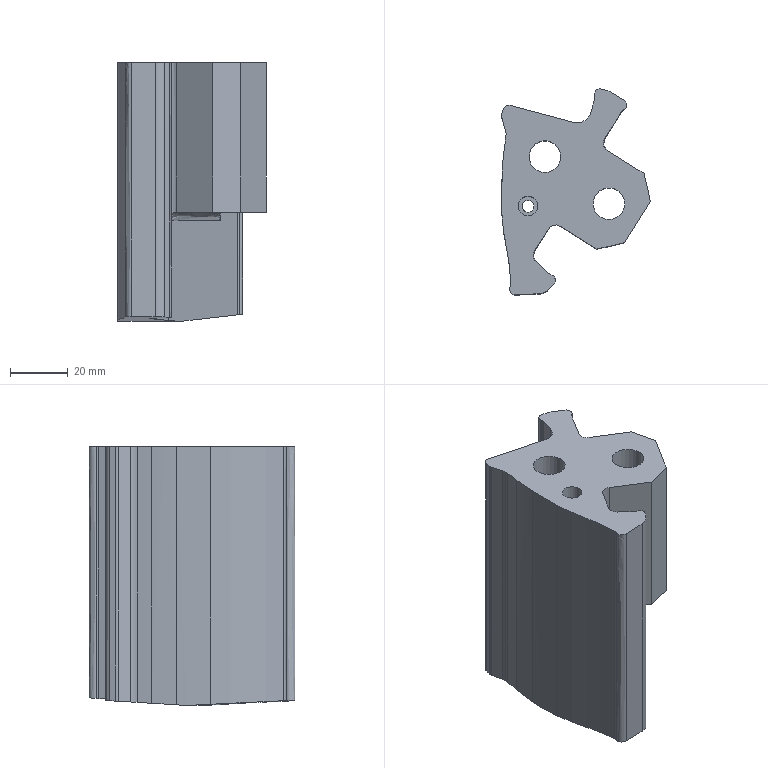Part | NX | features solid 2 | 1 solid | 52 faces | box 51.76 x 71.575 x 89.996 mm | volume 143214 mm3 | spline 24 | cylinder 15 | plane 13 | commonest cylinder face diameters 10 x4 4 x2 6 x2 11 x2 17 x2 4.1 x1